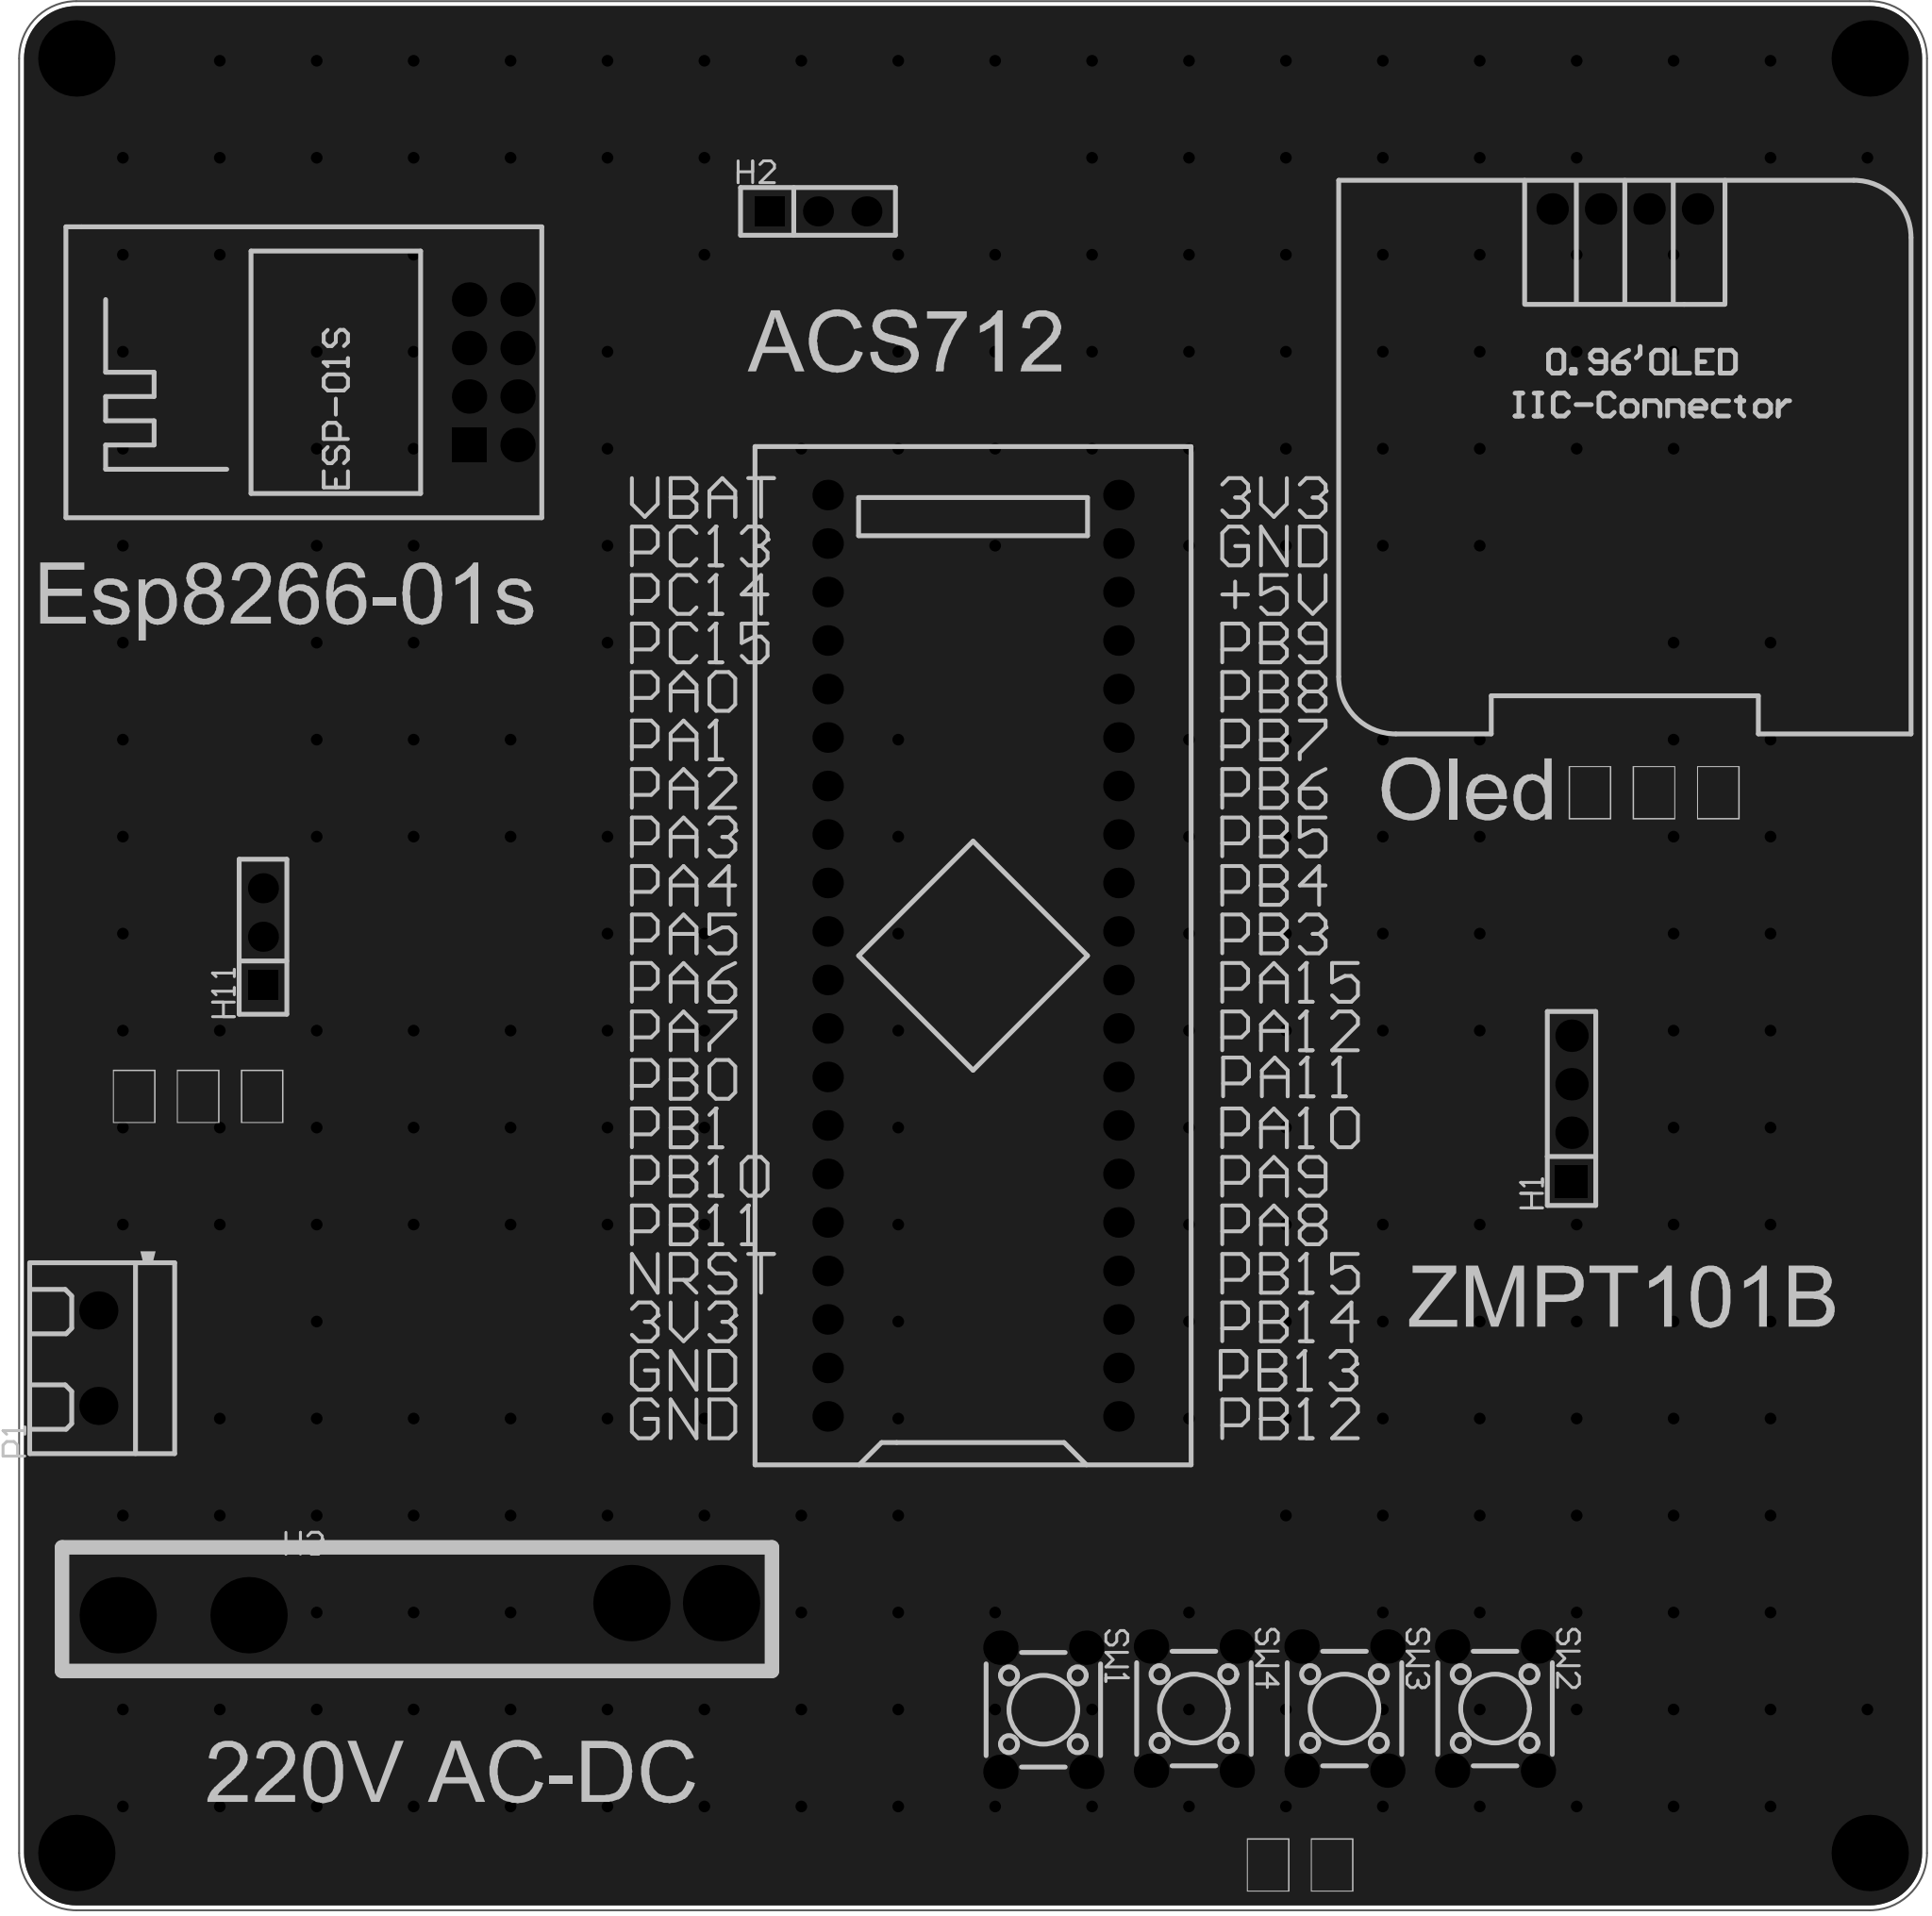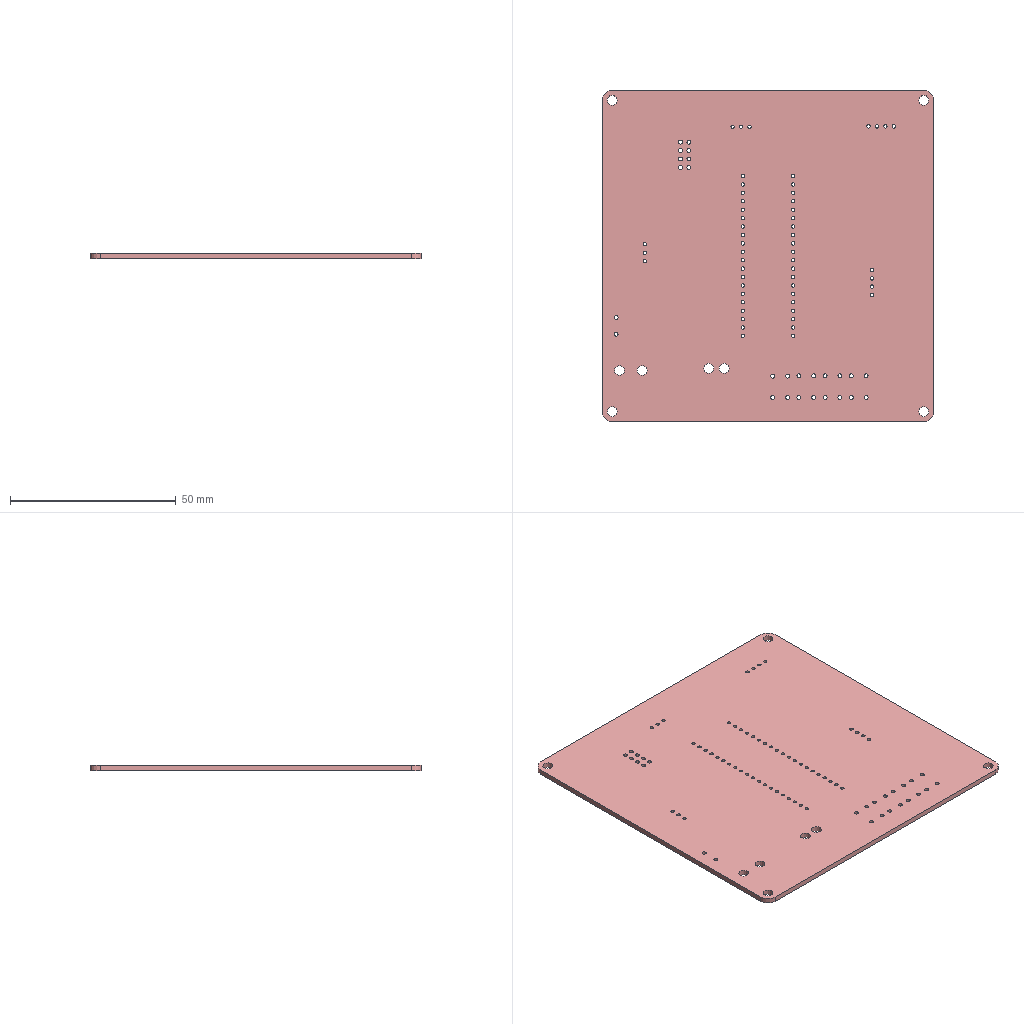Circuit board layout | Altium Designer | box 100 x 100 x 1.6 mm
Layer stack:
# Altium Designer layer stack of  (unit mm; dielectric type: 0 none, 1 core, 2 prepreg, 3 surface material)
index,name,kind,layer,copper_thickness_mm,dielectric_type,dielectric_thickness_mm,dielectric_material,dielectric_constant
0,Top Paste Mask Layer,other,,,,,,
1,Top Silkscreen Layer,other,,,,,,
2,Top Solder Mask Layer,dielectric,,,3,0.01,,3.3
3,Top Layer,copper,Top Layer,0.035,,,,
4,Dielectric1,dielectric,,,3,1.51,FR4,4.5
5,Bottom Layer,copper,Bottom Layer,0.035,,,,
6,Bottom Solder Mask Layer,dielectric,,,3,0.01,,3.3
7,Bottom Silkscreen Layer,other,,,,,,
8,Bottom Paste Mask Layer,other,,,,,,
# drill layer pairs: low layer,high layer
drill_pair,Top Layer,Bottom Layer
Part placement:
Designator,Comment,Layer,Footprint,Center-X(mm),Center-Y(mm),Rotation
U1,STM32F103C8T6-Card,TopLayer,CONN-TH_L53.3-W22.9_STM32F103C8T6-CARD,141.351,130.937,90
U2,ESP-01S,TopLayer,WIFIM-TH_ESP-01S,116.205,161.499,90
OLED1,,TopLayer,0.96OLED_4P,175.514,170.053,0
SW1,,TopLayer,SW-TH_4P-L6.0-W6.0-P4.50-LS6.5,145.034,91.44,270
SW2,,TopLayer,SW-TH_4P-L6.0-W6.0-P4.50-LS6.5,168.71,91.503,270
SW3,,TopLayer,SW-TH_4P-L6.0-W6.0-P4.50-LS6.5,160.818,91.503,270
SW4,,TopLayer,SW-TH_4P-L6.0-W6.0-P4.50-LS6.5,152.926,91.503,270
H11,,TopLayer,HDR-TH_3P-P2.54-V-F,104.133,131.931,90
H2,,TopLayer,HDR-TH_3P-P2.54-V-F,133.223,169.926,0
P1,KF301-2P接线端子,TopLayer,CONN-TH_XY301V-A-5.0-2P,95.504,109.855,90
H3,,TopLayer,HDR-TH_4P-P2.54-V-F,112.332,96.71,0
H1,,TopLayer,HDR-TH_4P-P2.54-V-M,172.72,122.936,90
Pad and via stacks:
# Altium Designer via and pad stacks of  (unit mm). Each distinct definition once, with the count of objects using it.
# via: kind,start_layer,end_layer,hole_mm,diameter_mm,mode(0 simple;1 top-mid-bottom;2 full stack),diameter_per_layer,count,example_net
# pad: kind,layer,hole_mm,hole_type(0 round;1 square;2 slot),plating,top_size,top_shape(1 round;2 rect;3 octagon;9 rounded rect),mid_size,bottom_size,mode,footprint,size_per_layer,count,example
pad,Multi-Layer,3,0,plated,4x4,1,4x4,4x4,0,,,4,1
pad,Multi-Layer,1,0,plated,1.6x1.6,1,1.6x1.6,1.6x1.6,0,CONN-TH_L53.3-W22.9_STM32F103C8T6-CARD,,40,U1.1
pad,Multi-Layer,1.2,0,plated,1.8x1.8,2,1.8x1.8,1.8x1.8,0,WIFIM-TH_ESP-01S,,1,U2.1
pad,Multi-Layer,1.2,0,plated,1.8x1.8,1,1.8x1.8,1.8x1.8,0,WIFIM-TH_ESP-01S,,7,U2.2
pad,Multi-Layer,1,0,plated,1.65x1.65,1,1.65x1.65,1.65x1.65,0,0.96OLED_4P,,4,OLED1.4
pad,Multi-Layer,1.2,0,plated,1.8x1.8,1,1.8x1.8,1.8x1.8,0,SW-TH_4P-L6.0-W6.0-P4.50-LS6.5,,16,SW1.1
pad,Multi-Layer,1.02,0,plated,1.575x1.575,1,1.575x1.575,1.575x1.575,0,HDR-TH_3P-P2.54-V-F,,4,H11.3
pad,Multi-Layer,1.02,0,plated,1.575x1.575,2,1.575x1.575,1.575x1.575,0,HDR-TH_3P-P2.54-V-F,,2,H11.1
pad,Multi-Layer,1.2,0,plated,2x2,1,2x2,2x2,0,CONN-TH_XY301V-A-5.0-2P,,2,P1.1
pad,Multi-Layer,3,0,plated,4x4,1,4x4,4x4,0,HDR-TH_4P-P2.54-V-F,,4,H3.1
pad,Multi-Layer,1.1,0,plated,1.7x1.7,2,1.7x1.7,1.7x1.7,0,HDR-TH_4P-P2.54-V-M,,1,H1.1
pad,Multi-Layer,1.1,0,plated,1.7x1.7,1,1.7x1.7,1.7x1.7,0,HDR-TH_4P-P2.54-V-M,,3,H1.2
via,Top Layer,Bottom Layer,0.3048,0.61,0,,248,GND
Copper pours:
name,layer,net,type(0 solid;1 hatched;2 none)
Bottom Layer-GND,Bottom Layer,GND,0
Top Layer-GND,Top Layer,GND,0